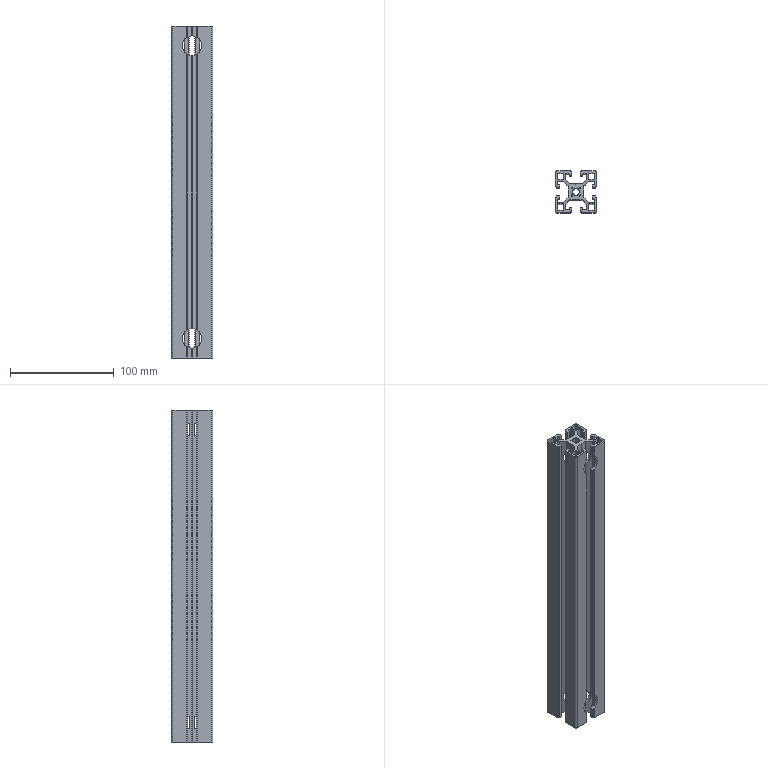Part | NX | features BREP 1 | 1 solid | 273 faces | box 40 x 40 x 320 mm | volume 187401 mm3 | plane 186 | cylinder 87 | commonest cylinder face diameters 1.5 x18 0.6 x16 2 x16 19 x16 6.8 x9 1 x8